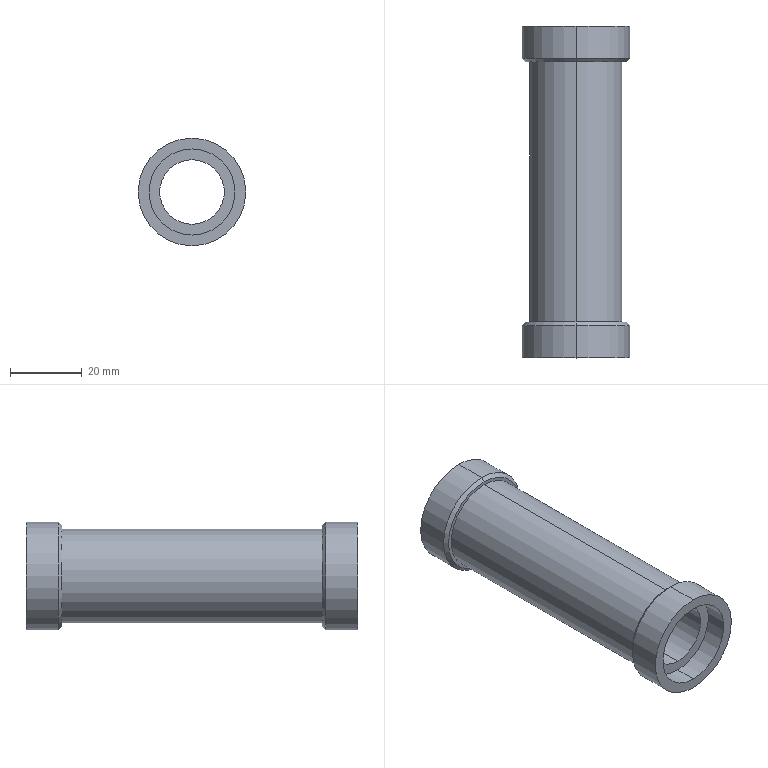Part | STEP file | 2012 Guide shaft | 1 solid | 22 faces | box 30 x 92.5 x 30 mm | volume 26584 mm3 | cylinder 12 | plane 6 | cone 4 | commonest cylinder face diameters 24 x4 30 x4 18 x2 26 x2
STEP:
#1=CARTESIAN_POINT('',(0.,0.,0.));
#2=DIRECTION('',(0.,0.,1.));
#3=DIRECTION('',(1.,0.,0.));
#4=AXIS2_PLACEMENT_3D('',#1,#2,#3);
#5=CARTESIAN_POINT('',(0.,82.5,-14.));
#6=VERTEX_POINT('',#5);
#7=CARTESIAN_POINT('',(0.,82.5,14.));
#8=VERTEX_POINT('',#7);
#9=CARTESIAN_POINT('',(0.,82.5,0.));
#10=DIRECTION('',(0.,-1.,0.));
#11=DIRECTION('',(0.,0.,-1.));
#12=AXIS2_PLACEMENT_3D('',#9,#10,#11);
#13=CIRCLE('',#12,14.);
#14=CARTESIAN_POINT('',(0.,82.5,0.));
#15=DIRECTION('',(0.,1.,0.));
#16=DIRECTION('',(0.,0.,1.));
#17=AXIS2_PLACEMENT_3D('',#14,#15,#16);
#18=CONICAL_SURFACE('',#17,14.,0.7854);
#19=CARTESIAN_POINT('',(3.142,0.));
#20=DIRECTION('',(-1.,0.));
#21=VECTOR('',#20,1.);
#22=LINE('',#19,#21);
#23=(GEOMETRIC_REPRESENTATION_CONTEXT(2)PARAMETRIC_REPRESENTATION_CONTEXT()REPRESENTATION_CONTEXT('',''));
#24=DEFINITIONAL_REPRESENTATION('',(#22),#23);
#25=PCURVE('',#18,#24);
#26=CARTESIAN_POINT('',(15.,82.5,0.));
#27=DIRECTION('',(0.,-1.,0.));
#28=DIRECTION('',(0.,0.,-1.));
#29=AXIS2_PLACEMENT_3D('',#26,#27,#28);
#30=PLANE('',#29);
#31=CARTESIAN_POINT('',(0.,-15.));
#32=DIRECTION('',(1.,0.));
#33=AXIS2_PLACEMENT_2D('',#31,#32);
#34=CIRCLE('',#33,14.);
#35=(GEOMETRIC_REPRESENTATION_CONTEXT(2)PARAMETRIC_REPRESENTATION_CONTEXT()REPRESENTATION_CONTEXT('',''));
#36=DEFINITIONAL_REPRESENTATION('',(#34),#35);
#37=PCURVE('',#30,#36);
#38=SURFACE_CURVE('',#13,(#25,#37),.PCURVE_S1.);
#39=EDGE_CURVE('',#6,#8,#38,.T.);
#40=ORIENTED_EDGE('',*,*,#39,.F.);
#41=CARTESIAN_POINT('',(0.,83.5,-15.));
#42=VERTEX_POINT('',#41);
#43=CARTESIAN_POINT('',(0.,82.5,-14.));
#44=DIRECTION('',(0.,0.7071,-0.7071));
#45=VECTOR('',#44,1.);
#46=LINE('',#43,#45);
#47=CARTESIAN_POINT('',(3.142,0.));
#48=DIRECTION('',(0.,1.));
#49=VECTOR('',#48,1.);
#50=LINE('',#47,#49);
#51=(GEOMETRIC_REPRESENTATION_CONTEXT(2)PARAMETRIC_REPRESENTATION_CONTEXT()REPRESENTATION_CONTEXT('',''));
#52=DEFINITIONAL_REPRESENTATION('',(#50),#51);
#53=PCURVE('',#18,#52);
#54=CARTESIAN_POINT('',(0.,82.5,0.));
#55=DIRECTION('',(0.,1.,0.));
#56=DIRECTION('',(0.,0.,1.));
#57=AXIS2_PLACEMENT_3D('',#54,#55,#56);
#58=CONICAL_SURFACE('',#57,14.,0.7854);
#59=CARTESIAN_POINT('',(3.142,0.));
#60=DIRECTION('',(0.,1.));
#61=VECTOR('',#60,1.);
#62=LINE('',#59,#61);
#63=(GEOMETRIC_REPRESENTATION_CONTEXT(2)PARAMETRIC_REPRESENTATION_CONTEXT()REPRESENTATION_CONTEXT('',''));
#64=DEFINITIONAL_REPRESENTATION('',(#62),#63);
#65=PCURVE('',#58,#64);
#66=SURFACE_CURVE('',#46,(#53,#65),.PCURVE_S1.);
#67=EDGE_CURVE('',#6,#42,#66,.T.);
#68=ORIENTED_EDGE('',*,*,#67,.T.);
#69=CARTESIAN_POINT('',(0.,83.5,15.));
#70=VERTEX_POINT('',#69);
#71=CARTESIAN_POINT('',(0.,83.5,0.));
#72=DIRECTION('',(0.,1.,0.));
#73=DIRECTION('',(0.,0.,-1.));
#74=AXIS2_PLACEMENT_3D('',#71,#72,#73);
#75=CIRCLE('',#74,15.);
#76=CARTESIAN_POINT('',(-3.142,1.));
#77=DIRECTION('',(1.,0.));
#78=VECTOR('',#77,1.);
#79=LINE('',#76,#78);
#80=(GEOMETRIC_REPRESENTATION_CONTEXT(2)PARAMETRIC_REPRESENTATION_CONTEXT()REPRESENTATION_CONTEXT('',''));
#81=DEFINITIONAL_REPRESENTATION('',(#79),#80);
#82=PCURVE('',#18,#81);
#83=CARTESIAN_POINT('',(0.,0.,0.));
#84=DIRECTION('',(0.,-1.,0.));
#85=DIRECTION('',(0.,0.,-1.));
#86=AXIS2_PLACEMENT_3D('',#83,#84,#85);
#87=CYLINDRICAL_SURFACE('',#86,15.);
#88=CARTESIAN_POINT('',(6.283,-83.5));
#89=DIRECTION('',(-1.,0.));
#90=VECTOR('',#89,1.);
#91=LINE('',#88,#90);
#92=(GEOMETRIC_REPRESENTATION_CONTEXT(2)PARAMETRIC_REPRESENTATION_CONTEXT()REPRESENTATION_CONTEXT('',''));
#93=DEFINITIONAL_REPRESENTATION('',(#91),#92);
#94=PCURVE('',#87,#93);
#95=SURFACE_CURVE('',#75,(#82,#94),.PCURVE_S1.);
#96=EDGE_CURVE('',#70,#42,#95,.T.);
#97=ORIENTED_EDGE('',*,*,#96,.F.);
#98=CARTESIAN_POINT('',(0.,82.5,14.));
#99=DIRECTION('',(0.,0.7071,0.7071));
#100=VECTOR('',#99,1.);
#101=LINE('',#98,#100);
#102=CARTESIAN_POINT('',(0.,0.));
#103=DIRECTION('',(0.,1.));
#104=VECTOR('',#103,1.);
#105=LINE('',#102,#104);
#106=(GEOMETRIC_REPRESENTATION_CONTEXT(2)PARAMETRIC_REPRESENTATION_CONTEXT()REPRESENTATION_CONTEXT('',''));
#107=DEFINITIONAL_REPRESENTATION('',(#105),#106);
#108=PCURVE('',#18,#107);
#109=CARTESIAN_POINT('',(6.283,0.));
#110=DIRECTION('',(0.,1.));
#111=VECTOR('',#110,1.);
#112=LINE('',#109,#111);
#113=(GEOMETRIC_REPRESENTATION_CONTEXT(2)PARAMETRIC_REPRESENTATION_CONTEXT()REPRESENTATION_CONTEXT('',''));
#114=DEFINITIONAL_REPRESENTATION('',(#112),#113);
#115=PCURVE('',#58,#114);
#116=SURFACE_CURVE('',#101,(#108,#115),.PCURVE_S1.);
#117=EDGE_CURVE('',#8,#70,#116,.T.);
#118=ORIENTED_EDGE('',*,*,#117,.F.);
#119=EDGE_LOOP('',(#40,#68,#97,#118));
#120=FACE_BOUND('',#119,.T.);
#121=ADVANCED_FACE('',(#120),#18,.T.);
#122=CARTESIAN_POINT('',(0.,10.,14.));
#123=VERTEX_POINT('',#122);
#124=CARTESIAN_POINT('',(0.,10.,-14.));
#125=VERTEX_POINT('',#124);
#126=CARTESIAN_POINT('',(0.,10.,0.));
#127=DIRECTION('',(0.,1.,0.));
#128=DIRECTION('',(0.,0.,1.));
#129=AXIS2_PLACEMENT_3D('',#126,#127,#128);
#130=CIRCLE('',#129,14.);
#131=CARTESIAN_POINT('',(0.,9.,0.));
#132=DIRECTION('',(0.,-1.,0.));
#133=DIRECTION('',(0.,0.,-1.));
#134=AXIS2_PLACEMENT_3D('',#131,#132,#133);
#135=CONICAL_SURFACE('',#134,15.,0.7854);
#136=CARTESIAN_POINT('',(3.142,-1.));
#137=DIRECTION('',(-1.,0.));
#138=VECTOR('',#137,1.);
#139=LINE('',#136,#138);
#140=(GEOMETRIC_REPRESENTATION_CONTEXT(2)PARAMETRIC_REPRESENTATION_CONTEXT()REPRESENTATION_CONTEXT('',''));
#141=DEFINITIONAL_REPRESENTATION('',(#139),#140);
#142=PCURVE('',#135,#141);
#143=CARTESIAN_POINT('',(13.,10.,0.));
#144=DIRECTION('',(0.,1.,0.));
#145=DIRECTION('',(0.,0.,1.));
#146=AXIS2_PLACEMENT_3D('',#143,#144,#145);
#147=PLANE('',#146);
#148=CARTESIAN_POINT('',(0.,-13.));
#149=DIRECTION('',(1.,0.));
#150=AXIS2_PLACEMENT_2D('',#148,#149);
#151=CIRCLE('',#150,14.);
#152=(GEOMETRIC_REPRESENTATION_CONTEXT(2)PARAMETRIC_REPRESENTATION_CONTEXT()REPRESENTATION_CONTEXT('',''));
#153=DEFINITIONAL_REPRESENTATION('',(#151),#152);
#154=PCURVE('',#147,#153);
#155=SURFACE_CURVE('',#130,(#142,#154),.PCURVE_S1.);
#156=EDGE_CURVE('',#123,#125,#155,.T.);
#157=ORIENTED_EDGE('',*,*,#156,.F.);
#158=CARTESIAN_POINT('',(0.,9.,15.));
#159=VERTEX_POINT('',#158);
#160=CARTESIAN_POINT('',(0.,9.,15.));
#161=DIRECTION('',(0.,-0.7071,0.7071));
#162=VECTOR('',#161,1.);
#163=LINE('',#160,#162);
#164=CARTESIAN_POINT('',(3.142,0.));
#165=DIRECTION('',(0.,1.));
#166=VECTOR('',#165,1.);
#167=LINE('',#164,#166);
#168=(GEOMETRIC_REPRESENTATION_CONTEXT(2)PARAMETRIC_REPRESENTATION_CONTEXT()REPRESENTATION_CONTEXT('',''));
#169=DEFINITIONAL_REPRESENTATION('',(#167),#168);
#170=PCURVE('',#135,#169);
#171=CARTESIAN_POINT('',(0.,9.,0.));
#172=DIRECTION('',(0.,-1.,0.));
#173=DIRECTION('',(0.,0.,-1.));
#174=AXIS2_PLACEMENT_3D('',#171,#172,#173);
#175=CONICAL_SURFACE('',#174,15.,0.7854);
#176=CARTESIAN_POINT('',(3.142,0.));
#177=DIRECTION('',(0.,1.));
#178=VECTOR('',#177,1.);
#179=LINE('',#176,#178);
#180=(GEOMETRIC_REPRESENTATION_CONTEXT(2)PARAMETRIC_REPRESENTATION_CONTEXT()REPRESENTATION_CONTEXT('',''));
#181=DEFINITIONAL_REPRESENTATION('',(#179),#180);
#182=PCURVE('',#175,#181);
#183=SURFACE_CURVE('',#163,(#170,#182),.PCURVE_S1.);
#184=EDGE_CURVE('',#123,#159,#183,.T.);
#185=ORIENTED_EDGE('',*,*,#184,.T.);
#186=CARTESIAN_POINT('',(0.,9.,-15.));
#187=VERTEX_POINT('',#186);
#188=CARTESIAN_POINT('',(0.,9.,0.));
#189=DIRECTION('',(0.,-1.,0.));
#190=DIRECTION('',(0.,0.,1.));
#191=AXIS2_PLACEMENT_3D('',#188,#189,#190);
#192=CIRCLE('',#191,15.);
#193=CARTESIAN_POINT('',(-3.142,0.));
#194=DIRECTION('',(1.,0.));
#195=VECTOR('',#194,1.);
#196=LINE('',#193,#195);
#197=(GEOMETRIC_REPRESENTATION_CONTEXT(2)PARAMETRIC_REPRESENTATION_CONTEXT()REPRESENTATION_CONTEXT('',''));
#198=DEFINITIONAL_REPRESENTATION('',(#196),#197);
#199=PCURVE('',#135,#198);
#200=CARTESIAN_POINT('',(0.,0.,0.));
#201=DIRECTION('',(0.,-1.,0.));
#202=DIRECTION('',(0.,0.,-1.));
#203=AXIS2_PLACEMENT_3D('',#200,#201,#202);
#204=CYLINDRICAL_SURFACE('',#203,15.);
#205=CARTESIAN_POINT('',(-3.142,-9.));
#206=DIRECTION('',(1.,0.));
#207=VECTOR('',#206,1.);
#208=LINE('',#205,#207);
#209=(GEOMETRIC_REPRESENTATION_CONTEXT(2)PARAMETRIC_REPRESENTATION_CONTEXT()REPRESENTATION_CONTEXT('',''));
#210=DEFINITIONAL_REPRESENTATION('',(#208),#209);
#211=PCURVE('',#204,#210);
#212=SURFACE_CURVE('',#192,(#199,#211),.PCURVE_S1.);
#213=EDGE_CURVE('',#187,#159,#212,.T.);
#214=ORIENTED_EDGE('',*,*,#213,.F.);
#215=CARTESIAN_POINT('',(0.,9.,-15.));
#216=DIRECTION('',(0.,-0.7071,-0.7071));
#217=VECTOR('',#216,1.);
#218=LINE('',#215,#217);
#219=CARTESIAN_POINT('',(0.,0.));
#220=DIRECTION('',(0.,1.));
#221=VECTOR('',#220,1.);
#222=LINE('',#219,#221);
#223=(GEOMETRIC_REPRESENTATION_CONTEXT(2)PARAMETRIC_REPRESENTATION_CONTEXT()REPRESENTATION_CONTEXT('',''));
#224=DEFINITIONAL_REPRESENTATION('',(#222),#223);
#225=PCURVE('',#135,#224);
#226=CARTESIAN_POINT('',(6.283,0.));
#227=DIRECTION('',(0.,1.));
#228=VECTOR('',#227,1.);
#229=LINE('',#226,#228);
#230=(GEOMETRIC_REPRESENTATION_CONTEXT(2)PARAMETRIC_REPRESENTATION_CONTEXT()REPRESENTATION_CONTEXT('',''));
#231=DEFINITIONAL_REPRESENTATION('',(#229),#230);
#232=PCURVE('',#175,#231);
#233=SURFACE_CURVE('',#218,(#225,#232),.PCURVE_S1.);
#234=EDGE_CURVE('',#125,#187,#233,.T.);
#235=ORIENTED_EDGE('',*,*,#234,.F.);
#236=EDGE_LOOP('',(#157,#185,#214,#235));
#237=FACE_BOUND('',#236,.T.);
#238=ADVANCED_FACE('',(#237),#135,.T.);
#239=CARTESIAN_POINT('',(0.,86.4,-9.));
#240=VERTEX_POINT('',#239);
#241=CARTESIAN_POINT('',(0.,6.1,-9.));
#242=VERTEX_POINT('',#241);
#243=CARTESIAN_POINT('',(0.,92.5,-9.));
#244=DIRECTION('',(0.,-1.,0.));
#245=VECTOR('',#244,1.);
#246=LINE('',#243,#245);
#247=CARTESIAN_POINT('',(0.,92.5,0.));
#248=DIRECTION('',(0.,-1.,0.));
#249=DIRECTION('',(0.,0.,-1.));
#250=AXIS2_PLACEMENT_3D('',#247,#248,#249);
#251=CYLINDRICAL_SURFACE('',#250,9.);
#252=CARTESIAN_POINT('',(6.283,0.));
#253=DIRECTION('',(0.,1.));
#254=VECTOR('',#253,1.);
#255=LINE('',#252,#254);
#256=(GEOMETRIC_REPRESENTATION_CONTEXT(2)PARAMETRIC_REPRESENTATION_CONTEXT()REPRESENTATION_CONTEXT('',''));
#257=DEFINITIONAL_REPRESENTATION('',(#255),#256);
#258=PCURVE('',#251,#257);
#259=CARTESIAN_POINT('',(0.,92.5,0.));
#260=DIRECTION('',(0.,-1.,0.));
#261=DIRECTION('',(0.,0.,-1.));
#262=AXIS2_PLACEMENT_3D('',#259,#260,#261);
#263=CYLINDRICAL_SURFACE('',#262,9.);
#264=CARTESIAN_POINT('',(0.,0.));
#265=DIRECTION('',(0.,1.));
#266=VECTOR('',#265,1.);
#267=LINE('',#264,#266);
#268=(GEOMETRIC_REPRESENTATION_CONTEXT(2)PARAMETRIC_REPRESENTATION_CONTEXT()REPRESENTATION_CONTEXT('',''));
#269=DEFINITIONAL_REPRESENTATION('',(#267),#268);
#270=PCURVE('',#263,#269);
#271=SURFACE_CURVE('',#246,(#258,#270),.PCURVE_S1.);
#272=EDGE_CURVE('',#240,#242,#271,.T.);
#273=ORIENTED_EDGE('',*,*,#272,.T.);
#274=CARTESIAN_POINT('',(0.,6.1,9.));
#275=VERTEX_POINT('',#274);
#276=CARTESIAN_POINT('',(0.,6.1,0.));
#277=DIRECTION('',(0.,-1.,0.));
#278=DIRECTION('',(0.,0.,-1.));
#279=AXIS2_PLACEMENT_3D('',#276,#277,#278);
#280=CIRCLE('',#279,9.);
#281=CARTESIAN_POINT('',(0.,86.4));
#282=DIRECTION('',(1.,0.));
#283=VECTOR('',#282,1.);
#284=LINE('',#281,#283);
#285=(GEOMETRIC_REPRESENTATION_CONTEXT(2)PARAMETRIC_REPRESENTATION_CONTEXT()REPRESENTATION_CONTEXT('',''));
#286=DEFINITIONAL_REPRESENTATION('',(#284),#285);
#287=PCURVE('',#251,#286);
#288=CARTESIAN_POINT('',(0.,6.1,0.));
#289=DIRECTION('',(0.,-1.,0.));
#290=DIRECTION('',(0.,0.,-1.));
#291=AXIS2_PLACEMENT_3D('',#288,#289,#290);
#292=PLANE('',#291);
#293=CARTESIAN_POINT('',(0.,0.));
#294=DIRECTION('',(1.,0.));
#295=AXIS2_PLACEMENT_2D('',#293,#294);
#296=CIRCLE('',#295,9.);
#297=(GEOMETRIC_REPRESENTATION_CONTEXT(2)PARAMETRIC_REPRESENTATION_CONTEXT()REPRESENTATION_CONTEXT('',''));
#298=DEFINITIONAL_REPRESENTATION('',(#296),#297);
#299=PCURVE('',#292,#298);
#300=SURFACE_CURVE('',#280,(#287,#299),.PCURVE_S1.);
#301=EDGE_CURVE('',#275,#242,#300,.T.);
#302=ORIENTED_EDGE('',*,*,#301,.F.);
#303=CARTESIAN_POINT('',(0.,86.4,9.));
#304=VERTEX_POINT('',#303);
#305=CARTESIAN_POINT('',(0.,92.5,9.));
#306=DIRECTION('',(0.,-1.,0.));
#307=VECTOR('',#306,1.);
#308=LINE('',#305,#307);
#309=CARTESIAN_POINT('',(3.142,0.));
#310=DIRECTION('',(0.,1.));
#311=VECTOR('',#310,1.);
#312=LINE('',#309,#311);
#313=(GEOMETRIC_REPRESENTATION_CONTEXT(2)PARAMETRIC_REPRESENTATION_CONTEXT()REPRESENTATION_CONTEXT('',''));
#314=DEFINITIONAL_REPRESENTATION('',(#312),#313);
#315=PCURVE('',#251,#314);
#316=CARTESIAN_POINT('',(3.142,0.));
#317=DIRECTION('',(0.,1.));
#318=VECTOR('',#317,1.);
#319=LINE('',#316,#318);
#320=(GEOMETRIC_REPRESENTATION_CONTEXT(2)PARAMETRIC_REPRESENTATION_CONTEXT()REPRESENTATION_CONTEXT('',''));
#321=DEFINITIONAL_REPRESENTATION('',(#319),#320);
#322=PCURVE('',#263,#321);
#323=SURFACE_CURVE('',#308,(#315,#322),.PCURVE_S1.);
#324=EDGE_CURVE('',#304,#275,#323,.T.);
#325=ORIENTED_EDGE('',*,*,#324,.F.);
#326=CARTESIAN_POINT('',(0.,86.4,0.));
#327=DIRECTION('',(0.,1.,0.));
#328=DIRECTION('',(0.,0.,1.));
#329=AXIS2_PLACEMENT_3D('',#326,#327,#328);
#330=CIRCLE('',#329,9.);
#331=CARTESIAN_POINT('',(9.425,6.1));
#332=DIRECTION('',(-1.,0.));
#333=VECTOR('',#332,1.);
#334=LINE('',#331,#333);
#335=(GEOMETRIC_REPRESENTATION_CONTEXT(2)PARAMETRIC_REPRESENTATION_CONTEXT()REPRESENTATION_CONTEXT('',''));
#336=DEFINITIONAL_REPRESENTATION('',(#334),#335);
#337=PCURVE('',#251,#336);
#338=CARTESIAN_POINT('',(0.,86.4,0.));
#339=DIRECTION('',(0.,1.,0.));
#340=DIRECTION('',(0.,0.,1.));
#341=AXIS2_PLACEMENT_3D('',#338,#339,#340);
#342=PLANE('',#341);
#343=CARTESIAN_POINT('',(0.,0.));
#344=DIRECTION('',(1.,0.));
#345=AXIS2_PLACEMENT_2D('',#343,#344);
#346=CIRCLE('',#345,9.);
#347=(GEOMETRIC_REPRESENTATION_CONTEXT(2)PARAMETRIC_REPRESENTATION_CONTEXT()REPRESENTATION_CONTEXT('',''));
#348=DEFINITIONAL_REPRESENTATION('',(#346),#347);
#349=PCURVE('',#342,#348);
#350=SURFACE_CURVE('',#330,(#337,#349),.PCURVE_S1.);
#351=EDGE_CURVE('',#240,#304,#350,.T.);
#352=ORIENTED_EDGE('',*,*,#351,.F.);
#353=EDGE_LOOP('',(#273,#302,#325,#352));
#354=FACE_BOUND('',#353,.F.);
#355=ADVANCED_FACE('',(#354),#251,.F.);
#356=CARTESIAN_POINT('',(0.,86.4,12.));
#357=VERTEX_POINT('',#356);
#358=CARTESIAN_POINT('',(0.,92.5,12.));
#359=VERTEX_POINT('',#358);
#360=CARTESIAN_POINT('',(0.,86.4,12.));
#361=DIRECTION('',(0.,1.,0.));
#362=VECTOR('',#361,1.);
#363=LINE('',#360,#362);
#364=CARTESIAN_POINT('',(0.,86.4,0.));
#365=DIRECTION('',(0.,1.,0.));
#366=DIRECTION('',(0.,0.,1.));
#367=AXIS2_PLACEMENT_3D('',#364,#365,#366);
#368=CYLINDRICAL_SURFACE('',#367,12.);
#369=CARTESIAN_POINT('',(6.283,0.));
#370=DIRECTION('',(0.,1.));
#371=VECTOR('',#370,1.);
#372=LINE('',#369,#371);
#373=(GEOMETRIC_REPRESENTATION_CONTEXT(2)PARAMETRIC_REPRESENTATION_CONTEXT()REPRESENTATION_CONTEXT('',''));
#374=DEFINITIONAL_REPRESENTATION('',(#372),#373);
#375=PCURVE('',#368,#374);
#376=CARTESIAN_POINT('',(0.,86.4,0.));
#377=DIRECTION('',(0.,1.,0.));
#378=DIRECTION('',(0.,0.,1.));
#379=AXIS2_PLACEMENT_3D('',#376,#377,#378);
#380=CYLINDRICAL_SURFACE('',#379,12.);
#381=CARTESIAN_POINT('',(0.,0.));
#382=DIRECTION('',(0.,1.));
#383=VECTOR('',#382,1.);
#384=LINE('',#381,#383);
#385=(GEOMETRIC_REPRESENTATION_CONTEXT(2)PARAMETRIC_REPRESENTATION_CONTEXT()REPRESENTATION_CONTEXT('',''));
#386=DEFINITIONAL_REPRESENTATION('',(#384),#385);
#387=PCURVE('',#380,#386);
#388=SURFACE_CURVE('',#363,(#375,#387),.PCURVE_S1.);
#389=EDGE_CURVE('',#357,#359,#388,.T.);
#390=ORIENTED_EDGE('',*,*,#389,.T.);
#391=CARTESIAN_POINT('',(0.,92.5,-12.));
#392=VERTEX_POINT('',#391);
#393=CARTESIAN_POINT('',(0.,92.5,0.));
#394=DIRECTION('',(0.,1.,0.));
#395=DIRECTION('',(0.,0.,1.));
#396=AXIS2_PLACEMENT_3D('',#393,#394,#395);
#397=CIRCLE('',#396,12.);
#398=CARTESIAN_POINT('',(0.,6.1));
#399=DIRECTION('',(1.,0.));
#400=VECTOR('',#399,1.);
#401=LINE('',#398,#400);
#402=(GEOMETRIC_REPRESENTATION_CONTEXT(2)PARAMETRIC_REPRESENTATION_CONTEXT()REPRESENTATION_CONTEXT('',''));
#403=DEFINITIONAL_REPRESENTATION('',(#401),#402);
#404=PCURVE('',#368,#403);
#405=CARTESIAN_POINT('',(0.,92.5,0.));
#406=DIRECTION('',(0.,1.,0.));
#407=DIRECTION('',(0.,0.,1.));
#408=AXIS2_PLACEMENT_3D('',#405,#406,#407);
#409=PLANE('',#408);
#410=CARTESIAN_POINT('',(0.,0.));
#411=DIRECTION('',(1.,0.));
#412=AXIS2_PLACEMENT_2D('',#410,#411);
#413=CIRCLE('',#412,12.);
#414=(GEOMETRIC_REPRESENTATION_CONTEXT(2)PARAMETRIC_REPRESENTATION_CONTEXT()REPRESENTATION_CONTEXT('',''));
#415=DEFINITIONAL_REPRESENTATION('',(#413),#414);
#416=PCURVE('',#409,#415);
#417=SURFACE_CURVE('',#397,(#404,#416),.PCURVE_S1.);
#418=EDGE_CURVE('',#392,#359,#417,.T.);
#419=ORIENTED_EDGE('',*,*,#418,.F.);
#420=CARTESIAN_POINT('',(0.,86.4,-12.));
#421=VERTEX_POINT('',#420);
#422=CARTESIAN_POINT('',(0.,86.4,-12.));
#423=DIRECTION('',(0.,1.,0.));
#424=VECTOR('',#423,1.);
#425=LINE('',#422,#424);
#426=CARTESIAN_POINT('',(3.142,0.));
#427=DIRECTION('',(0.,1.));
#428=VECTOR('',#427,1.);
#429=LINE('',#426,#428);
#430=(GEOMETRIC_REPRESENTATION_CONTEXT(2)PARAMETRIC_REPRESENTATION_CONTEXT()REPRESENTATION_CONTEXT('',''));
#431=DEFINITIONAL_REPRESENTATION('',(#429),#430);
#432=PCURVE('',#368,#431);
#433=CARTESIAN_POINT('',(3.142,0.));
#434=DIRECTION('',(0.,1.));
#435=VECTOR('',#434,1.);
#436=LINE('',#433,#435);
#437=(GEOMETRIC_REPRESENTATION_CONTEXT(2)PARAMETRIC_REPRESENTATION_CONTEXT()REPRESENTATION_CONTEXT('',''));
#438=DEFINITIONAL_REPRESENTATION('',(#436),#437);
#439=PCURVE('',#380,#438);
#440=SURFACE_CURVE('',#425,(#432,#439),.PCURVE_S1.);
#441=EDGE_CURVE('',#421,#392,#440,.T.);
#442=ORIENTED_EDGE('',*,*,#441,.F.);
#443=CARTESIAN_POINT('',(0.,86.4,0.));
#444=DIRECTION('',(0.,1.,0.));
#445=DIRECTION('',(0.,0.,1.));
#446=AXIS2_PLACEMENT_3D('',#443,#444,#445);
#447=CIRCLE('',#446,12.);
#448=CARTESIAN_POINT('',(0.,0.));
#449=DIRECTION('',(1.,0.));
#450=VECTOR('',#449,1.);
#451=LINE('',#448,#450);
#452=(GEOMETRIC_REPRESENTATION_CONTEXT(2)PARAMETRIC_REPRESENTATION_CONTEXT()REPRESENTATION_CONTEXT('',''));
#453=DEFINITIONAL_REPRESENTATION('',(#451),#452);
#454=PCURVE('',#368,#453);
#455=CARTESIAN_POINT('',(0.,0.));
#456=DIRECTION('',(1.,0.));
#457=AXIS2_PLACEMENT_2D('',#455,#456);
#458=CIRCLE('',#457,12.);
#459=(GEOMETRIC_REPRESENTATION_CONTEXT(2)PARAMETRIC_REPRESENTATION_CONTEXT()REPRESENTATION_CONTEXT('',''));
#460=DEFINITIONAL_REPRESENTATION('',(#458),#459);
#461=PCURVE('',#342,#460);
#462=SURFACE_CURVE('',#447,(#454,#461),.PCURVE_S1.);
#463=EDGE_CURVE('',#421,#357,#462,.T.);
#464=ORIENTED_EDGE('',*,*,#463,.T.);
#465=EDGE_LOOP('',(#390,#419,#442,#464));
#466=FACE_BOUND('',#465,.F.);
#467=ADVANCED_FACE('',(#466),#368,.F.);
#468=CARTESIAN_POINT('',(0.,6.1,-12.));
#469=VERTEX_POINT('',#468);
#470=CARTESIAN_POINT('',(0.,0.,-12.));
#471=VERTEX_POINT('',#470);
#472=CARTESIAN_POINT('',(0.,6.1,-12.));
#473=DIRECTION('',(0.,-1.,0.));
#474=VECTOR('',#473,1.);
#475=LINE('',#472,#474);
#476=CARTESIAN_POINT('',(0.,6.1,0.));
#477=DIRECTION('',(0.,-1.,0.));
#478=DIRECTION('',(0.,0.,-1.));
#479=AXIS2_PLACEMENT_3D('',#476,#477,#478);
#480=CYLINDRICAL_SURFACE('',#479,12.);
#481=CARTESIAN_POINT('',(6.283,0.));
#482=DIRECTION('',(0.,1.));
#483=VECTOR('',#482,1.);
#484=LINE('',#481,#483);
#485=(GEOMETRIC_REPRESENTATION_CONTEXT(2)PARAMETRIC_REPRESENTATION_CONTEXT()REPRESENTATION_CONTEXT('',''));
#486=DEFINITIONAL_REPRESENTATION('',(#484),#485);
#487=PCURVE('',#480,#486);
#488=CARTESIAN_POINT('',(0.,6.1,0.));
#489=DIRECTION('',(0.,-1.,0.));
#490=DIRECTION('',(0.,0.,-1.));
#491=AXIS2_PLACEMENT_3D('',#488,#489,#490);
#492=CYLINDRICAL_SURFACE('',#491,12.);
#493=CARTESIAN_POINT('',(0.,0.));
#494=DIRECTION('',(0.,1.));
#495=VECTOR('',#494,1.);
#496=LINE('',#493,#495);
#497=(GEOMETRIC_REPRESENTATION_CONTEXT(2)PARAMETRIC_REPRESENTATION_CONTEXT()REPRESENTATION_CONTEXT('',''));
#498=DEFINITIONAL_REPRESENTATION('',(#496),#497);
#499=PCURVE('',#492,#498);
#500=SURFACE_CURVE('',#475,(#487,#499),.PCURVE_S1.);
#501=EDGE_CURVE('',#469,#471,#500,.T.);
#502=ORIENTED_EDGE('',*,*,#501,.T.);
#503=CARTESIAN_POINT('',(0.,0.,12.));
#504=VERTEX_POINT('',#503);
#505=CARTESIAN_POINT('',(0.,0.,0.));
#506=DIRECTION('',(0.,-1.,0.));
#507=DIRECTION('',(0.,0.,-1.));
#508=AXIS2_PLACEMENT_3D('',#505,#506,#507);
#509=CIRCLE('',#508,12.);
#510=CARTESIAN_POINT('',(0.,6.1));
#511=DIRECTION('',(1.,0.));
#512=VECTOR('',#511,1.);
#513=LINE('',#510,#512);
#514=(GEOMETRIC_REPRESENTATION_CONTEXT(2)PARAMETRIC_REPRESENTATION_CONTEXT()REPRESENTATION_CONTEXT('',''));
#515=DEFINITIONAL_REPRESENTATION('',(#513),#514);
#516=PCURVE('',#480,#515);
#517=CARTESIAN_POINT('',(15.,0.,0.));
#518=DIRECTION('',(0.,-1.,0.));
#519=DIRECTION('',(0.,0.,-1.));
#520=AXIS2_PLACEMENT_3D('',#517,#518,#519);
#521=PLANE('',#520);
#522=CARTESIAN_POINT('',(0.,-15.));
#523=DIRECTION('',(1.,0.));
#524=AXIS2_PLACEMENT_2D('',#522,#523);
#525=CIRCLE('',#524,12.);
#526=(GEOMETRIC_REPRESENTATION_CONTEXT(2)PARAMETRIC_REPRESENTATION_CONTEXT()REPRESENTATION_CONTEXT('',''));
#527=DEFINITIONAL_REPRESENTATION('',(#525),#526);
#528=PCURVE('',#521,#527);
#529=SURFACE_CURVE('',#509,(#516,#528),.PCURVE_S1.);
#530=EDGE_CURVE('',#504,#471,#529,.T.);
#531=ORIENTED_EDGE('',*,*,#530,.F.);
#532=CARTESIAN_POINT('',(0.,6.1,12.));
#533=VERTEX_POINT('',#532);
#534=CARTESIAN_POINT('',(0.,6.1,12.));
#535=DIRECTION('',(0.,-1.,0.));
#536=VECTOR('',#535,1.);
#537=LINE('',#534,#536);
#538=CARTESIAN_POINT('',(3.142,0.));
#539=DIRECTION('',(0.,1.));
#540=VECTOR('',#539,1.);
#541=LINE('',#538,#540);
#542=(GEOMETRIC_REPRESENTATION_CONTEXT(2)PARAMETRIC_REPRESENTATION_CONTEXT()REPRESENTATION_CONTEXT('',''));
#543=DEFINITIONAL_REPRESENTATION('',(#541),#542);
#544=PCURVE('',#480,#543);
#545=CARTESIAN_POINT('',(3.142,0.));
#546=DIRECTION('',(0.,1.));
#547=VECTOR('',#546,1.);
#548=LINE('',#545,#547);
#549=(GEOMETRIC_REPRESENTATION_CONTEXT(2)PARAMETRIC_REPRESENTATION_CONTEXT()REPRESENTATION_CONTEXT('',''));
#550=DEFINITIONAL_REPRESENTATION('',(#548),#549);
#551=PCURVE('',#492,#550);
#552=SURFACE_CURVE('',#537,(#544,#551),.PCURVE_S1.);
#553=EDGE_CURVE('',#533,#504,#552,.T.);
#554=ORIENTED_EDGE('',*,*,#553,.F.);
#555=CARTESIAN_POINT('',(0.,6.1,0.));
#556=DIRECTION('',(0.,-1.,0.));
#557=DIRECTION('',(0.,0.,-1.));
#558=AXIS2_PLACEMENT_3D('',#555,#556,#557);
#559=CIRCLE('',#558,12.);
#560=CARTESIAN_POINT('',(0.,0.));
#561=DIRECTION('',(1.,0.));
#562=VECTOR('',#561,1.);
#563=LINE('',#560,#562);
#564=(GEOMETRIC_REPRESENTATION_CONTEXT(2)PARAMETRIC_REPRESENTATION_CONTEXT()REPRESENTATION_CONTEXT('',''));
#565=DEFINITIONAL_REPRESENTATION('',(#563),#564);
#566=PCURVE('',#480,#565);
#567=CARTESIAN_POINT('',(0.,0.));
#568=DIRECTION('',(1.,0.));
#569=AXIS2_PLACEMENT_2D('',#567,#568);
#570=CIRCLE('',#569,12.);
#571=(GEOMETRIC_REPRESENTATION_CONTEXT(2)PARAMETRIC_REPRESENTATION_CONTEXT()REPRESENTATION_CONTEXT('',''));
#572=DEFINITIONAL_REPRESENTATION('',(#570),#571);
#573=PCURVE('',#292,#572);
#574=SURFACE_CURVE('',#559,(#566,#573),.PCURVE_S1.);
#575=EDGE_CURVE('',#533,#469,#574,.T.);
#576=ORIENTED_EDGE('',*,*,#575,.T.);
#577=EDGE_LOOP('',(#502,#531,#554,#576));
#578=FACE_BOUND('',#577,.F.);
#579=ADVANCED_FACE('',(#578),#480,.F.);
#580=ORIENTED_EDGE('',*,*,#213,.T.);
#581=CARTESIAN_POINT('',(0.,0.,15.));
#582=VERTEX_POINT('',#581);
#583=CARTESIAN_POINT('',(0.,0.,15.));
#584=DIRECTION('',(0.,-1.,0.));
#585=VECTOR('',#584,1.);
#586=LINE('',#583,#585);
#587=CARTESIAN_POINT('',(3.142,0.));
#588=DIRECTION('',(0.,1.));
#589=VECTOR('',#588,1.);
#590=LINE('',#587,#589);
#591=(GEOMETRIC_REPRESENTATION_CONTEXT(2)PARAMETRIC_REPRESENTATION_CONTEXT()REPRESENTATION_CONTEXT('',''));
#592=DEFINITIONAL_REPRESENTATION('',(#590),#591);
#593=PCURVE('',#204,#592);
#594=CARTESIAN_POINT('',(0.,0.,0.));
#595=DIRECTION('',(0.,-1.,0.));
#596=DIRECTION('',(0.,0.,-1.));
#597=AXIS2_PLACEMENT_3D('',#594,#595,#596);
#598=CYLINDRICAL_SURFACE('',#597,15.);
#599=CARTESIAN_POINT('',(3.142,0.));
#600=DIRECTION('',(0.,1.));
#601=VECTOR('',#600,1.);
#602=LINE('',#599,#601);
#603=(GEOMETRIC_REPRESENTATION_CONTEXT(2)PARAMETRIC_REPRESENTATION_CONTEXT()REPRESENTATION_CONTEXT('',''));
#604=DEFINITIONAL_REPRESENTATION('',(#602),#603);
#605=PCURVE('',#598,#604);
#606=SURFACE_CURVE('',#586,(#593,#605),.PCURVE_S1.);
#607=EDGE_CURVE('',#159,#582,#606,.T.);
#608=ORIENTED_EDGE('',*,*,#607,.T.);
#609=CARTESIAN_POINT('',(0.,0.,-15.));
#610=VERTEX_POINT('',#609);
#611=CARTESIAN_POINT('',(0.,0.,0.));
#612=DIRECTION('',(0.,-1.,0.));
#613=DIRECTION('',(0.,0.,-1.));
#614=AXIS2_PLACEMENT_3D('',#611,#612,#613);
#615=CIRCLE('',#614,15.);
#616=CARTESIAN_POINT('',(0.,0.));
#617=DIRECTION('',(1.,0.));
#618=VECTOR('',#617,1.);
#619=LINE('',#616,#618);
#620=(GEOMETRIC_REPRESENTATION_CONTEXT(2)PARAMETRIC_REPRESENTATION_CONTEXT()REPRESENTATION_CONTEXT('',''));
#621=DEFINITIONAL_REPRESENTATION('',(#619),#620);
#622=PCURVE('',#204,#621);
#623=CARTESIAN_POINT('',(0.,-15.));
#624=DIRECTION('',(1.,0.));
#625=AXIS2_PLACEMENT_2D('',#623,#624);
#626=CIRCLE('',#625,15.);
#627=(GEOMETRIC_REPRESENTATION_CONTEXT(2)PARAMETRIC_REPRESENTATION_CONTEXT()REPRESENTATION_CONTEXT('',''));
#628=DEFINITIONAL_REPRESENTATION('',(#626),#627);
#629=PCURVE('',#521,#628);
#630=SURFACE_CURVE('',#615,(#622,#629),.PCURVE_S1.);
#631=EDGE_CURVE('',#610,#582,#630,.T.);
#632=ORIENTED_EDGE('',*,*,#631,.F.);
#633=CARTESIAN_POINT('',(0.,0.,-15.));
#634=DIRECTION('',(0.,-1.,0.));
#635=VECTOR('',#634,1.);
#636=LINE('',#633,#635);
#637=CARTESIAN_POINT('',(0.,0.));
#638=DIRECTION('',(0.,1.));
#639=VECTOR('',#638,1.);
#640=LINE('',#637,#639);
#641=(GEOMETRIC_REPRESENTATION_CONTEXT(2)PARAMETRIC_REPRESENTATION_CONTEXT()REPRESENTATION_CONTEXT('',''));
#642=DEFINITIONAL_REPRESENTATION('',(#640),#641);
#643=PCURVE('',#204,#642);
#644=CARTESIAN_POINT('',(6.283,0.));
#645=DIRECTION('',(0.,1.));
#646=VECTOR('',#645,1.);
#647=LINE('',#644,#646);
#648=(GEOMETRIC_REPRESENTATION_CONTEXT(2)PARAMETRIC_REPRESENTATION_CONTEXT()REPRESENTATION_CONTEXT('',''));
#649=DEFINITIONAL_REPRESENTATION('',(#647),#648);
#650=PCURVE('',#598,#649);
#651=SURFACE_CURVE('',#636,(#643,#650),.PCURVE_S1.);
#652=EDGE_CURVE('',#187,#610,#651,.T.);
#653=ORIENTED_EDGE('',*,*,#652,.F.);
#654=EDGE_LOOP('',(#580,#608,#632,#653));
#655=FACE_BOUND('',#654,.T.);
#656=ADVANCED_FACE('',(#655),#204,.T.);
#657=CARTESIAN_POINT('',(0.,82.5,-13.));
#658=VERTEX_POINT('',#657);
#659=CARTESIAN_POINT('',(0.,82.5,13.));
#660=VERTEX_POINT('',#659);
#661=CARTESIAN_POINT('',(0.,82.5,0.));
#662=DIRECTION('',(0.,-1.,0.));
#663=DIRECTION('',(0.,0.,-1.));
#664=AXIS2_PLACEMENT_3D('',#661,#662,#663);
#665=CIRCLE('',#664,13.);
#666=CARTESIAN_POINT('',(0.,0.,0.));
#667=DIRECTION('',(0.,-1.,0.));
#668=DIRECTION('',(0.,0.,-1.));
#669=AXIS2_PLACEMENT_3D('',#666,#667,#668);
#670=CYLINDRICAL_SURFACE('',#669,13.);
#671=CARTESIAN_POINT('',(0.,-82.5));
#672=DIRECTION('',(1.,0.));
#673=VECTOR('',#672,1.);
#674=LINE('',#671,#673);
#675=(GEOMETRIC_REPRESENTATION_CONTEXT(2)PARAMETRIC_REPRESENTATION_CONTEXT()REPRESENTATION_CONTEXT('',''));
#676=DEFINITIONAL_REPRESENTATION('',(#674),#675);
#677=PCURVE('',#670,#676);
#678=CARTESIAN_POINT('',(0.,-15.));
#679=DIRECTION('',(1.,0.));
#680=AXIS2_PLACEMENT_2D('',#678,#679);
#681=CIRCLE('',#680,13.);
#682=(GEOMETRIC_REPRESENTATION_CONTEXT(2)PARAMETRIC_REPRESENTATION_CONTEXT()REPRESENTATION_CONTEXT('',''));
#683=DEFINITIONAL_REPRESENTATION('',(#681),#682);
#684=PCURVE('',#30,#683);
#685=SURFACE_CURVE('',#665,(#677,#684),.PCURVE_S1.);
#686=EDGE_CURVE('',#658,#660,#685,.T.);
#687=ORIENTED_EDGE('',*,*,#686,.T.);
#688=CARTESIAN_POINT('',(0.,10.,13.));
#689=VERTEX_POINT('',#688);
#690=CARTESIAN_POINT('',(0.,0.,13.));
#691=DIRECTION('',(0.,-1.,0.));
#692=VECTOR('',#691,1.);
#693=LINE('',#690,#692);
#694=CARTESIAN_POINT('',(3.142,0.));
#695=DIRECTION('',(0.,1.));
#696=VECTOR('',#695,1.);
#697=LINE('',#694,#696);
#698=(GEOMETRIC_REPRESENTATION_CONTEXT(2)PARAMETRIC_REPRESENTATION_CONTEXT()REPRESENTATION_CONTEXT('',''));
#699=DEFINITIONAL_REPRESENTATION('',(#697),#698);
#700=PCURVE('',#670,#699);
#701=CARTESIAN_POINT('',(0.,0.,0.));
#702=DIRECTION('',(0.,-1.,0.));
#703=DIRECTION('',(0.,0.,-1.));
#704=AXIS2_PLACEMENT_3D('',#701,#702,#703);
#705=CYLINDRICAL_SURFACE('',#704,13.);
#706=CARTESIAN_POINT('',(3.142,0.));
#707=DIRECTION('',(0.,1.));
#708=VECTOR('',#707,1.);
#709=LINE('',#706,#708);
#710=(GEOMETRIC_REPRESENTATION_CONTEXT(2)PARAMETRIC_REPRESENTATION_CONTEXT()REPRESENTATION_CONTEXT('',''));
#711=DEFINITIONAL_REPRESENTATION('',(#709),#710);
#712=PCURVE('',#705,#711);
#713=SURFACE_CURVE('',#693,(#700,#712),.PCURVE_S1.);
#714=EDGE_CURVE('',#660,#689,#713,.T.);
#715=ORIENTED_EDGE('',*,*,#714,.T.);
#716=CARTESIAN_POINT('',(0.,10.,-13.));
#717=VERTEX_POINT('',#716);
#718=CARTESIAN_POINT('',(0.,10.,0.));
#719=DIRECTION('',(0.,-1.,0.));
#720=DIRECTION('',(0.,0.,-1.));
#721=AXIS2_PLACEMENT_3D('',#718,#719,#720);
#722=CIRCLE('',#721,13.);
#723=CARTESIAN_POINT('',(0.,-10.));
#724=DIRECTION('',(1.,0.));
#725=VECTOR('',#724,1.);
#726=LINE('',#723,#725);
#727=(GEOMETRIC_REPRESENTATION_CONTEXT(2)PARAMETRIC_REPRESENTATION_CONTEXT()REPRESENTATION_CONTEXT('',''));
#728=DEFINITIONAL_REPRESENTATION('',(#726),#727);
#729=PCURVE('',#670,#728);
#730=CARTESIAN_POINT('',(-13.,-13.));
#731=CARTESIAN_POINT('',(-13.,9.517));
#732=CARTESIAN_POINT('',(6.5,-1.742));
#733=CARTESIAN_POINT('',(26.,-13.));
#734=CARTESIAN_POINT('',(6.5,-24.258));
#735=CARTESIAN_POINT('',(-13.,-35.517));
#736=CARTESIAN_POINT('',(-13.,-13.));
#737=(BOUNDED_CURVE()B_SPLINE_CURVE(2,(#730,#731,#732,#733,#734,#735,#736),.UNSPECIFIED.,.T.,.F.)B_SPLINE_CURVE_WITH_KNOTS((1,2,2,2,2,1),(-2.094,0.,2.094,4.189,6.283,8.378),.UNSPECIFIED.)CURVE()GEOMETRIC_REPRESENTATION_ITEM()RATIONAL_B_SPLINE_CURVE((1.,0.5,1.,0.5,1.,0.5,1.))REPRESENTATION_ITEM(''));
#738=(GEOMETRIC_REPRESENTATION_CONTEXT(2)PARAMETRIC_REPRESENTATION_CONTEXT()REPRESENTATION_CONTEXT('',''));
#739=DEFINITIONAL_REPRESENTATION('',(#737),#738);
#740=PCURVE('',#147,#739);
#741=SURFACE_CURVE('',#722,(#729,#740),.PCURVE_S1.);
#742=EDGE_CURVE('',#717,#689,#741,.T.);
#743=ORIENTED_EDGE('',*,*,#742,.F.);
#744=CARTESIAN_POINT('',(0.,0.,-13.));
#745=DIRECTION('',(0.,-1.,0.));
#746=VECTOR('',#745,1.);
#747=LINE('',#744,#746);
#748=CARTESIAN_POINT('',(0.,0.));
#749=DIRECTION('',(0.,1.));
#750=VECTOR('',#749,1.);
#751=LINE('',#748,#750);
#752=(GEOMETRIC_REPRESENTATION_CONTEXT(2)PARAMETRIC_REPRESENTATION_CONTEXT()REPRESENTATION_CONTEXT('',''));
#753=DEFINITIONAL_REPRESENTATION('',(#751),#752);
#754=PCURVE('',#670,#753);
#755=CARTESIAN_POINT('',(6.283,0.));
#756=DIRECTION('',(0.,1.));
#757=VECTOR('',#756,1.);
#758=LINE('',#755,#757);
#759=(GEOMETRIC_REPRESENTATION_CONTEXT(2)PARAMETRIC_REPRESENTATION_CONTEXT()REPRESENTATION_CONTEXT('',''));
#760=DEFINITIONAL_REPRESENTATION('',(#758),#759);
#761=PCURVE('',#705,#760);
#762=SURFACE_CURVE('',#747,(#754,#761),.PCURVE_S1.);
#763=EDGE_CURVE('',#658,#717,#762,.T.);
#764=ORIENTED_EDGE('',*,*,#763,.F.);
#765=EDGE_LOOP('',(#687,#715,#743,#764));
#766=FACE_BOUND('',#765,.T.);
#767=ADVANCED_FACE('',(#766),#670,.T.);
#768=CARTESIAN_POINT('',(0.,92.5,-15.));
#769=VERTEX_POINT('',#768);
#770=CARTESIAN_POINT('',(0.,92.5,15.));
#771=VERTEX_POINT('',#770);
#772=CARTESIAN_POINT('',(0.,92.5,0.));
#773=DIRECTION('',(0.,-1.,0.));
#774=DIRECTION('',(0.,0.,-1.));
#775=AXIS2_PLACEMENT_3D('',#772,#773,#774);
#776=CIRCLE('',#775,15.);
#777=CARTESIAN_POINT('',(0.,-92.5));
#778=DIRECTION('',(1.,0.));
#779=VECTOR('',#778,1.);
#780=LINE('',#777,#779);
#781=(GEOMETRIC_REPRESENTATION_CONTEXT(2)PARAMETRIC_REPRESENTATION_CONTEXT()REPRESENTATION_CONTEXT('',''));
#782=DEFINITIONAL_REPRESENTATION('',(#780),#781);
#783=PCURVE('',#87,#782);
#784=CARTESIAN_POINT('',(-15.,0.));
#785=CARTESIAN_POINT('',(-15.,25.981));
#786=CARTESIAN_POINT('',(7.5,12.99));
#787=CARTESIAN_POINT('',(30.,0.));
#788=CARTESIAN_POINT('',(7.5,-12.99));
#789=CARTESIAN_POINT('',(-15.,-25.981));
#790=CARTESIAN_POINT('',(-15.,0.));
#791=(BOUNDED_CURVE()B_SPLINE_CURVE(2,(#784,#785,#786,#787,#788,#789,#790),.UNSPECIFIED.,.T.,.F.)B_SPLINE_CURVE_WITH_KNOTS((1,2,2,2,2,1),(-2.094,0.,2.094,4.189,6.283,8.378),.UNSPECIFIED.)CURVE()GEOMETRIC_REPRESENTATION_ITEM()RATIONAL_B_SPLINE_CURVE((1.,0.5,1.,0.5,1.,0.5,1.))REPRESENTATION_ITEM(''));
#792=(GEOMETRIC_REPRESENTATION_CONTEXT(2)PARAMETRIC_REPRESENTATION_CONTEXT()REPRESENTATION_CONTEXT('',''));
#793=DEFINITIONAL_REPRESENTATION('',(#791),#792);
#794=PCURVE('',#409,#793);
#795=SURFACE_CURVE('',#776,(#783,#794),.PCURVE_S1.);
#796=EDGE_CURVE('',#769,#771,#795,.T.);
#797=ORIENTED_EDGE('',*,*,#796,.T.);
#798=CARTESIAN_POINT('',(0.,0.,15.));
#799=DIRECTION('',(0.,-1.,0.));
#800=VECTOR('',#799,1.);
#801=LINE('',#798,#800);
#802=CARTESIAN_POINT('',(3.142,0.));
#803=DIRECTION('',(0.,1.));
#804=VECTOR('',#803,1.);
#805=LINE('',#802,#804);
#806=(GEOMETRIC_REPRESENTATION_CONTEXT(2)PARAMETRIC_REPRESENTATION_CONTEXT()REPRESENTATION_CONTEXT('',''));
#807=DEFINITIONAL_REPRESENTATION('',(#805),#806);
#808=PCURVE('',#87,#807);
#809=CARTESIAN_POINT('',(0.,0.,0.));
#810=DIRECTION('',(0.,-1.,0.));
#811=DIRECTION('',(0.,0.,-1.));
#812=AXIS2_PLACEMENT_3D('',#809,#810,#811);
#813=CYLINDRICAL_SURFACE('',#812,15.);
#814=CARTESIAN_POINT('',(3.142,0.));
#815=DIRECTION('',(0.,1.));
#816=VECTOR('',#815,1.);
#817=LINE('',#814,#816);
#818=(GEOMETRIC_REPRESENTATION_CONTEXT(2)PARAMETRIC_REPRESENTATION_CONTEXT()REPRESENTATION_CONTEXT('',''));
#819=DEFINITIONAL_REPRESENTATION('',(#817),#818);
#820=PCURVE('',#813,#819);
#821=SURFACE_CURVE('',#801,(#808,#820),.PCURVE_S1.);
#822=EDGE_CURVE('',#771,#70,#821,.T.);
#823=ORIENTED_EDGE('',*,*,#822,.T.);
#824=ORIENTED_EDGE('',*,*,#96,.T.);
#825=CARTESIAN_POINT('',(0.,0.,-15.));
#826=DIRECTION('',(0.,-1.,0.));
#827=VECTOR('',#826,1.);
#828=LINE('',#825,#827);
#829=CARTESIAN_POINT('',(0.,0.));
#830=DIRECTION('',(0.,1.));
#831=VECTOR('',#830,1.);
#832=LINE('',#829,#831);
#833=(GEOMETRIC_REPRESENTATION_CONTEXT(2)PARAMETRIC_REPRESENTATION_CONTEXT()REPRESENTATION_CONTEXT('',''));
#834=DEFINITIONAL_REPRESENTATION('',(#832),#833);
#835=PCURVE('',#87,#834);
#836=CARTESIAN_POINT('',(6.283,0.));
#837=DIRECTION('',(0.,1.));
#838=VECTOR('',#837,1.);
#839=LINE('',#836,#838);
#840=(GEOMETRIC_REPRESENTATION_CONTEXT(2)PARAMETRIC_REPRESENTATION_CONTEXT()REPRESENTATION_CONTEXT('',''));
#841=DEFINITIONAL_REPRESENTATION('',(#839),#840);
#842=PCURVE('',#813,#841);
#843=SURFACE_CURVE('',#828,(#835,#842),.PCURVE_S1.);
#844=EDGE_CURVE('',#769,#42,#843,.T.);
#845=ORIENTED_EDGE('',*,*,#844,.F.);
#846=EDGE_LOOP('',(#797,#823,#824,#845));
#847=FACE_BOUND('',#846,.T.);
#848=ADVANCED_FACE('',(#847),#87,.T.);
#849=CARTESIAN_POINT('',(0.,0.,0.));
#850=DIRECTION('',(0.,-1.,0.));
#851=DIRECTION('',(0.,0.,-1.));
#852=AXIS2_PLACEMENT_3D('',#849,#850,#851);
#853=CIRCLE('',#852,12.);
#854=CARTESIAN_POINT('',(0.,-15.));
#855=DIRECTION('',(1.,0.));
#856=AXIS2_PLACEMENT_2D('',#854,#855);
#857=CIRCLE('',#856,12.);
#858=(GEOMETRIC_REPRESENTATION_CONTEXT(2)PARAMETRIC_REPRESENTATION_CONTEXT()REPRESENTATION_CONTEXT('',''));
#859=DEFINITIONAL_REPRESENTATION('',(#857),#858);
#860=PCURVE('',#521,#859);
#861=CARTESIAN_POINT('',(0.,6.1));
#862=DIRECTION('',(1.,0.));
#863=VECTOR('',#862,1.);
#864=LINE('',#861,#863);
#865=(GEOMETRIC_REPRESENTATION_CONTEXT(2)PARAMETRIC_REPRESENTATION_CONTEXT()REPRESENTATION_CONTEXT('',''));
#866=DEFINITIONAL_REPRESENTATION('',(#864),#865);
#867=PCURVE('',#492,#866);
#868=SURFACE_CURVE('',#853,(#860,#867),.PCURVE_S1.);
#869=EDGE_CURVE('',#471,#504,#868,.T.);
#870=ORIENTED_EDGE('',*,*,#869,.F.);
#871=ORIENTED_EDGE('',*,*,#530,.F.);
#872=EDGE_LOOP('',(#870,#871));
#873=FACE_BOUND('',#872,.T.);
#874=ORIENTED_EDGE('',*,*,#631,.T.);
#875=CARTESIAN_POINT('',(0.,0.,0.));
#876=DIRECTION('',(0.,-1.,0.));
#877=DIRECTION('',(0.,0.,-1.));
#878=AXIS2_PLACEMENT_3D('',#875,#876,#877);
#879=CIRCLE('',#878,15.);
#880=CARTESIAN_POINT('',(0.,-15.));
#881=DIRECTION('',(1.,0.));
#882=AXIS2_PLACEMENT_2D('',#880,#881);
#883=CIRCLE('',#882,15.);
#884=(GEOMETRIC_REPRESENTATION_CONTEXT(2)PARAMETRIC_REPRESENTATION_CONTEXT()REPRESENTATION_CONTEXT('',''));
#885=DEFINITIONAL_REPRESENTATION('',(#883),#884);
#886=PCURVE('',#521,#885);
#887=CARTESIAN_POINT('',(0.,0.));
#888=DIRECTION('',(1.,0.));
#889=VECTOR('',#888,1.);
#890=LINE('',#887,#889);
#891=(GEOMETRIC_REPRESENTATION_CONTEXT(2)PARAMETRIC_REPRESENTATION_CONTEXT()REPRESENTATION_CONTEXT('',''));
#892=DEFINITIONAL_REPRESENTATION('',(#890),#891);
#893=PCURVE('',#598,#892);
#894=SURFACE_CURVE('',#879,(#886,#893),.PCURVE_S1.);
#895=EDGE_CURVE('',#582,#610,#894,.T.);
#896=ORIENTED_EDGE('',*,*,#895,.T.);
#897=EDGE_LOOP('',(#874,#896));
#898=FACE_BOUND('',#897,.T.);
#899=ADVANCED_FACE('',(#873,#898),#521,.T.);
#900=CARTESIAN_POINT('',(0.,92.5,0.));
#901=DIRECTION('',(0.,1.,0.));
#902=DIRECTION('',(0.,0.,1.));
#903=AXIS2_PLACEMENT_3D('',#900,#901,#902);
#904=CIRCLE('',#903,12.);
#905=CARTESIAN_POINT('',(0.,0.));
#906=DIRECTION('',(1.,0.));
#907=AXIS2_PLACEMENT_2D('',#905,#906);
#908=CIRCLE('',#907,12.);
#909=(GEOMETRIC_REPRESENTATION_CONTEXT(2)PARAMETRIC_REPRESENTATION_CONTEXT()REPRESENTATION_CONTEXT('',''));
#910=DEFINITIONAL_REPRESENTATION('',(#908),#909);
#911=PCURVE('',#409,#910);
#912=CARTESIAN_POINT('',(0.,6.1));
#913=DIRECTION('',(1.,0.));
#914=VECTOR('',#913,1.);
#915=LINE('',#912,#914);
#916=(GEOMETRIC_REPRESENTATION_CONTEXT(2)PARAMETRIC_REPRESENTATION_CONTEXT()REPRESENTATION_CONTEXT('',''));
#917=DEFINITIONAL_REPRESENTATION('',(#915),#916);
#918=PCURVE('',#380,#917);
#919=SURFACE_CURVE('',#904,(#911,#918),.PCURVE_S1.);
#920=EDGE_CURVE('',#359,#392,#919,.T.);
#921=ORIENTED_EDGE('',*,*,#920,.F.);
#922=ORIENTED_EDGE('',*,*,#418,.F.);
#923=EDGE_LOOP('',(#921,#922));
#924=FACE_BOUND('',#923,.T.);
#925=ORIENTED_EDGE('',*,*,#796,.F.);
#926=CARTESIAN_POINT('',(0.,92.5,0.));
#927=DIRECTION('',(0.,-1.,0.));
#928=DIRECTION('',(0.,0.,-1.));
#929=AXIS2_PLACEMENT_3D('',#926,#927,#928);
#930=CIRCLE('',#929,15.);
#931=CARTESIAN_POINT('',(-15.,0.));
#932=CARTESIAN_POINT('',(-15.,25.981));
#933=CARTESIAN_POINT('',(7.5,12.99));
#934=CARTESIAN_POINT('',(30.,0.));
#935=CARTESIAN_POINT('',(7.5,-12.99));
#936=CARTESIAN_POINT('',(-15.,-25.981));
#937=CARTESIAN_POINT('',(-15.,0.));
#938=(BOUNDED_CURVE()B_SPLINE_CURVE(2,(#931,#932,#933,#934,#935,#936,#937),.UNSPECIFIED.,.T.,.F.)B_SPLINE_CURVE_WITH_KNOTS((1,2,2,2,2,1),(-2.094,0.,2.094,4.189,6.283,8.378),.UNSPECIFIED.)CURVE()GEOMETRIC_REPRESENTATION_ITEM()RATIONAL_B_SPLINE_CURVE((1.,0.5,1.,0.5,1.,0.5,1.))REPRESENTATION_ITEM(''));
#939=(GEOMETRIC_REPRESENTATION_CONTEXT(2)PARAMETRIC_REPRESENTATION_CONTEXT()REPRESENTATION_CONTEXT('',''));
#940=DEFINITIONAL_REPRESENTATION('',(#938),#939);
#941=PCURVE('',#409,#940);
#942=CARTESIAN_POINT('',(0.,-92.5));
#943=DIRECTION('',(1.,0.));
#944=VECTOR('',#943,1.);
#945=LINE('',#942,#944);
#946=(GEOMETRIC_REPRESENTATION_CONTEXT(2)PARAMETRIC_REPRESENTATION_CONTEXT()REPRESENTATION_CONTEXT('',''));
#947=DEFINITIONAL_REPRESENTATION('',(#945),#946);
#948=PCURVE('',#813,#947);
#949=SURFACE_CURVE('',#930,(#941,#948),.PCURVE_S1.);
#950=EDGE_CURVE('',#771,#769,#949,.T.);
#951=ORIENTED_EDGE('',*,*,#950,.F.);
#952=EDGE_LOOP('',(#925,#951));
#953=FACE_BOUND('',#952,.T.);
#954=ADVANCED_FACE('',(#924,#953),#409,.T.);
#955=ORIENTED_EDGE('',*,*,#822,.F.);
#956=ORIENTED_EDGE('',*,*,#950,.T.);
#957=ORIENTED_EDGE('',*,*,#844,.T.);
#958=CARTESIAN_POINT('',(0.,83.5,0.));
#959=DIRECTION('',(0.,1.,0.));
#960=DIRECTION('',(0.,0.,-1.));
#961=AXIS2_PLACEMENT_3D('',#958,#959,#960);
#962=CIRCLE('',#961,15.);
#963=CARTESIAN_POINT('',(6.283,-83.5));
#964=DIRECTION('',(-1.,0.));
#965=VECTOR('',#964,1.);
#966=LINE('',#963,#965);
#967=(GEOMETRIC_REPRESENTATION_CONTEXT(2)PARAMETRIC_REPRESENTATION_CONTEXT()REPRESENTATION_CONTEXT('',''));
#968=DEFINITIONAL_REPRESENTATION('',(#966),#967);
#969=PCURVE('',#813,#968);
#970=CARTESIAN_POINT('',(3.142,1.));
#971=DIRECTION('',(1.,0.));
#972=VECTOR('',#971,1.);
#973=LINE('',#970,#972);
#974=(GEOMETRIC_REPRESENTATION_CONTEXT(2)PARAMETRIC_REPRESENTATION_CONTEXT()REPRESENTATION_CONTEXT('',''));
#975=DEFINITIONAL_REPRESENTATION('',(#973),#974);
#976=PCURVE('',#58,#975);
#977=SURFACE_CURVE('',#962,(#969,#976),.PCURVE_S1.);
#978=EDGE_CURVE('',#42,#70,#977,.T.);
#979=ORIENTED_EDGE('',*,*,#978,.T.);
#980=EDGE_LOOP('',(#955,#956,#957,#979));
#981=FACE_BOUND('',#980,.T.);
#982=ADVANCED_FACE('',(#981),#813,.T.);
#983=CARTESIAN_POINT('',(0.,82.5,0.));
#984=DIRECTION('',(0.,-1.,0.));
#985=DIRECTION('',(0.,0.,-1.));
#986=AXIS2_PLACEMENT_3D('',#983,#984,#985);
#987=CIRCLE('',#986,14.);
#988=CARTESIAN_POINT('',(0.,-15.));
#989=DIRECTION('',(1.,0.));
#990=AXIS2_PLACEMENT_2D('',#988,#989);
#991=CIRCLE('',#990,14.);
#992=(GEOMETRIC_REPRESENTATION_CONTEXT(2)PARAMETRIC_REPRESENTATION_CONTEXT()REPRESENTATION_CONTEXT('',''));
#993=DEFINITIONAL_REPRESENTATION('',(#991),#992);
#994=PCURVE('',#30,#993);
#995=CARTESIAN_POINT('',(9.425,0.));
#996=DIRECTION('',(-1.,0.));
#997=VECTOR('',#996,1.);
#998=LINE('',#995,#997);
#999=(GEOMETRIC_REPRESENTATION_CONTEXT(2)PARAMETRIC_REPRESENTATION_CONTEXT()REPRESENTATION_CONTEXT('',''));
#1000=DEFINITIONAL_REPRESENTATION('',(#998),#999);
#1001=PCURVE('',#58,#1000);
#1002=SURFACE_CURVE('',#987,(#994,#1001),.PCURVE_S1.);
#1003=EDGE_CURVE('',#8,#6,#1002,.T.);
#1004=ORIENTED_EDGE('',*,*,#1003,.T.);
#1005=ORIENTED_EDGE('',*,*,#39,.T.);
#1006=EDGE_LOOP('',(#1004,#1005));
#1007=FACE_BOUND('',#1006,.T.);
#1008=ORIENTED_EDGE('',*,*,#686,.F.);
#1009=CARTESIAN_POINT('',(0.,82.5,0.));
#1010=DIRECTION('',(0.,-1.,0.));
#1011=DIRECTION('',(0.,0.,-1.));
#1012=AXIS2_PLACEMENT_3D('',#1009,#1010,#1011);
#1013=CIRCLE('',#1012,13.);
#1014=CARTESIAN_POINT('',(0.,-15.));
#1015=DIRECTION('',(1.,0.));
#1016=AXIS2_PLACEMENT_2D('',#1014,#1015);
#1017=CIRCLE('',#1016,13.);
#1018=(GEOMETRIC_REPRESENTATION_CONTEXT(2)PARAMETRIC_REPRESENTATION_CONTEXT()REPRESENTATION_CONTEXT('',''));
#1019=DEFINITIONAL_REPRESENTATION('',(#1017),#1018);
#1020=PCURVE('',#30,#1019);
#1021=CARTESIAN_POINT('',(0.,-82.5));
#1022=DIRECTION('',(1.,0.));
#1023=VECTOR('',#1022,1.);
#1024=LINE('',#1021,#1023);
#1025=(GEOMETRIC_REPRESENTATION_CONTEXT(2)PARAMETRIC_REPRESENTATION_CONTEXT()REPRESENTATION_CONTEXT('',''));
#1026=DEFINITIONAL_REPRESENTATION('',(#1024),#1025);
#1027=PCURVE('',#705,#1026);
#1028=SURFACE_CURVE('',#1013,(#1020,#1027),.PCURVE_S1.);
#1029=EDGE_CURVE('',#660,#658,#1028,.T.);
#1030=ORIENTED_EDGE('',*,*,#1029,.F.);
#1031=EDGE_LOOP('',(#1008,#1030));
#1032=FACE_BOUND('',#1031,.T.);
#1033=ADVANCED_FACE('',(#1007,#1032),#30,.T.);
#1034=ORIENTED_EDGE('',*,*,#714,.F.);
#1035=ORIENTED_EDGE('',*,*,#1029,.T.);
#1036=ORIENTED_EDGE('',*,*,#763,.T.);
#1037=CARTESIAN_POINT('',(0.,10.,0.));
#1038=DIRECTION('',(0.,-1.,0.));
#1039=DIRECTION('',(0.,0.,-1.));
#1040=AXIS2_PLACEMENT_3D('',#1037,#1038,#1039);
#1041=CIRCLE('',#1040,13.);
#1042=CARTESIAN_POINT('',(0.,-10.));
#1043=DIRECTION('',(1.,0.));
#1044=VECTOR('',#1043,1.);
#1045=LINE('',#1042,#1044);
#1046=(GEOMETRIC_REPRESENTATION_CONTEXT(2)PARAMETRIC_REPRESENTATION_CONTEXT()REPRESENTATION_CONTEXT('',''));
#1047=DEFINITIONAL_REPRESENTATION('',(#1045),#1046);
#1048=PCURVE('',#705,#1047);
#1049=CARTESIAN_POINT('',(-13.,-13.));
#1050=CARTESIAN_POINT('',(-13.,9.517));
#1051=CARTESIAN_POINT('',(6.5,-1.742));
#1052=CARTESIAN_POINT('',(26.,-13.));
#1053=CARTESIAN_POINT('',(6.5,-24.258));
#1054=CARTESIAN_POINT('',(-13.,-35.517));
#1055=CARTESIAN_POINT('',(-13.,-13.));
#1056=(BOUNDED_CURVE()B_SPLINE_CURVE(2,(#1049,#1050,#1051,#1052,#1053,#1054,#1055),.UNSPECIFIED.,.T.,.F.)B_SPLINE_CURVE_WITH_KNOTS((1,2,2,2,2,1),(-2.094,0.,2.094,4.189,6.283,8.378),.UNSPECIFIED.)CURVE()GEOMETRIC_REPRESENTATION_ITEM()RATIONAL_B_SPLINE_CURVE((1.,0.5,1.,0.5,1.,0.5,1.))REPRESENTATION_ITEM(''));
#1057=(GEOMETRIC_REPRESENTATION_CONTEXT(2)PARAMETRIC_REPRESENTATION_CONTEXT()REPRESENTATION_CONTEXT('',''));
#1058=DEFINITIONAL_REPRESENTATION('',(#1056),#1057);
#1059=PCURVE('',#147,#1058);
#1060=SURFACE_CURVE('',#1041,(#1048,#1059),.PCURVE_S1.);
#1061=EDGE_CURVE('',#689,#717,#1060,.T.);
#1062=ORIENTED_EDGE('',*,*,#1061,.F.);
#1063=EDGE_LOOP('',(#1034,#1035,#1036,#1062));
#1064=FACE_BOUND('',#1063,.T.);
#1065=ADVANCED_FACE('',(#1064),#705,.T.);
#1066=CARTESIAN_POINT('',(0.,10.,0.));
#1067=DIRECTION('',(0.,1.,0.));
#1068=DIRECTION('',(0.,0.,1.));
#1069=AXIS2_PLACEMENT_3D('',#1066,#1067,#1068);
#1070=CIRCLE('',#1069,14.);
#1071=CARTESIAN_POINT('',(0.,-13.));
#1072=DIRECTION('',(1.,0.));
#1073=AXIS2_PLACEMENT_2D('',#1071,#1072);
#1074=CIRCLE('',#1073,14.);
#1075=(GEOMETRIC_REPRESENTATION_CONTEXT(2)PARAMETRIC_REPRESENTATION_CONTEXT()REPRESENTATION_CONTEXT('',''));
#1076=DEFINITIONAL_REPRESENTATION('',(#1074),#1075);
#1077=PCURVE('',#147,#1076);
#1078=CARTESIAN_POINT('',(9.425,-1.));
#1079=DIRECTION('',(-1.,0.));
#1080=VECTOR('',#1079,1.);
#1081=LINE('',#1078,#1080);
#1082=(GEOMETRIC_REPRESENTATION_CONTEXT(2)PARAMETRIC_REPRESENTATION_CONTEXT()REPRESENTATION_CONTEXT('',''));
#1083=DEFINITIONAL_REPRESENTATION('',(#1081),#1082);
#1084=PCURVE('',#175,#1083);
#1085=SURFACE_CURVE('',#1070,(#1077,#1084),.PCURVE_S1.);
#1086=EDGE_CURVE('',#125,#123,#1085,.T.);
#1087=ORIENTED_EDGE('',*,*,#1086,.T.);
#1088=ORIENTED_EDGE('',*,*,#156,.T.);
#1089=EDGE_LOOP('',(#1087,#1088));
#1090=FACE_BOUND('',#1089,.T.);
#1091=ORIENTED_EDGE('',*,*,#742,.T.);
#1092=ORIENTED_EDGE('',*,*,#1061,.T.);
#1093=EDGE_LOOP('',(#1091,#1092));
#1094=FACE_BOUND('',#1093,.T.);
#1095=ADVANCED_FACE('',(#1090,#1094),#147,.T.);
#1096=ORIENTED_EDGE('',*,*,#607,.F.);
#1097=CARTESIAN_POINT('',(0.,9.,0.));
#1098=DIRECTION('',(0.,-1.,0.));
#1099=DIRECTION('',(0.,0.,1.));
#1100=AXIS2_PLACEMENT_3D('',#1097,#1098,#1099);
#1101=CIRCLE('',#1100,15.);
#1102=CARTESIAN_POINT('',(3.142,-9.));
#1103=DIRECTION('',(1.,0.));
#1104=VECTOR('',#1103,1.);
#1105=LINE('',#1102,#1104);
#1106=(GEOMETRIC_REPRESENTATION_CONTEXT(2)PARAMETRIC_REPRESENTATION_CONTEXT()REPRESENTATION_CONTEXT('',''));
#1107=DEFINITIONAL_REPRESENTATION('',(#1105),#1106);
#1108=PCURVE('',#598,#1107);
#1109=CARTESIAN_POINT('',(3.142,0.));
#1110=DIRECTION('',(1.,0.));
#1111=VECTOR('',#1110,1.);
#1112=LINE('',#1109,#1111);
#1113=(GEOMETRIC_REPRESENTATION_CONTEXT(2)PARAMETRIC_REPRESENTATION_CONTEXT()REPRESENTATION_CONTEXT('',''));
#1114=DEFINITIONAL_REPRESENTATION('',(#1112),#1113);
#1115=PCURVE('',#175,#1114);
#1116=SURFACE_CURVE('',#1101,(#1108,#1115),.PCURVE_S1.);
#1117=EDGE_CURVE('',#159,#187,#1116,.T.);
#1118=ORIENTED_EDGE('',*,*,#1117,.T.);
#1119=ORIENTED_EDGE('',*,*,#652,.T.);
#1120=ORIENTED_EDGE('',*,*,#895,.F.);
#1121=EDGE_LOOP('',(#1096,#1118,#1119,#1120));
#1122=FACE_BOUND('',#1121,.T.);
#1123=ADVANCED_FACE('',(#1122),#598,.T.);
#1124=ORIENTED_EDGE('',*,*,#869,.F.);
#1125=ORIENTED_EDGE('',*,*,#501,.F.);
#1126=CARTESIAN_POINT('',(0.,6.1,0.));
#1127=DIRECTION('',(0.,-1.,0.));
#1128=DIRECTION('',(0.,0.,-1.));
#1129=AXIS2_PLACEMENT_3D('',#1126,#1127,#1128);
#1130=CIRCLE('',#1129,12.);
#1131=CARTESIAN_POINT('',(0.,0.));
#1132=DIRECTION('',(1.,0.));
#1133=VECTOR('',#1132,1.);
#1134=LINE('',#1131,#1133);
#1135=(GEOMETRIC_REPRESENTATION_CONTEXT(2)PARAMETRIC_REPRESENTATION_CONTEXT()REPRESENTATION_CONTEXT('',''));
#1136=DEFINITIONAL_REPRESENTATION('',(#1134),#1135);
#1137=PCURVE('',#492,#1136);
#1138=CARTESIAN_POINT('',(0.,0.));
#1139=DIRECTION('',(1.,0.));
#1140=AXIS2_PLACEMENT_2D('',#1138,#1139);
#1141=CIRCLE('',#1140,12.);
#1142=(GEOMETRIC_REPRESENTATION_CONTEXT(2)PARAMETRIC_REPRESENTATION_CONTEXT()REPRESENTATION_CONTEXT('',''));
#1143=DEFINITIONAL_REPRESENTATION('',(#1141),#1142);
#1144=PCURVE('',#292,#1143);
#1145=SURFACE_CURVE('',#1130,(#1137,#1144),.PCURVE_S1.);
#1146=EDGE_CURVE('',#469,#533,#1145,.T.);
#1147=ORIENTED_EDGE('',*,*,#1146,.T.);
#1148=ORIENTED_EDGE('',*,*,#553,.T.);
#1149=EDGE_LOOP('',(#1124,#1125,#1147,#1148));
#1150=FACE_BOUND('',#1149,.F.);
#1151=ADVANCED_FACE('',(#1150),#492,.F.);
#1152=CARTESIAN_POINT('',(0.,6.1,0.));
#1153=DIRECTION('',(0.,-1.,0.));
#1154=DIRECTION('',(0.,0.,-1.));
#1155=AXIS2_PLACEMENT_3D('',#1152,#1153,#1154);
#1156=CIRCLE('',#1155,9.);
#1157=CARTESIAN_POINT('',(0.,0.));
#1158=DIRECTION('',(1.,0.));
#1159=AXIS2_PLACEMENT_2D('',#1157,#1158);
#1160=CIRCLE('',#1159,9.);
#1161=(GEOMETRIC_REPRESENTATION_CONTEXT(2)PARAMETRIC_REPRESENTATION_CONTEXT()REPRESENTATION_CONTEXT('',''));
#1162=DEFINITIONAL_REPRESENTATION('',(#1160),#1161);
#1163=PCURVE('',#292,#1162);
#1164=CARTESIAN_POINT('',(0.,86.4));
#1165=DIRECTION('',(1.,0.));
#1166=VECTOR('',#1165,1.);
#1167=LINE('',#1164,#1166);
#1168=(GEOMETRIC_REPRESENTATION_CONTEXT(2)PARAMETRIC_REPRESENTATION_CONTEXT()REPRESENTATION_CONTEXT('',''));
#1169=DEFINITIONAL_REPRESENTATION('',(#1167),#1168);
#1170=PCURVE('',#263,#1169);
#1171=SURFACE_CURVE('',#1156,(#1163,#1170),.PCURVE_S1.);
#1172=EDGE_CURVE('',#242,#275,#1171,.T.);
#1173=ORIENTED_EDGE('',*,*,#1172,.F.);
#1174=ORIENTED_EDGE('',*,*,#301,.F.);
#1175=EDGE_LOOP('',(#1173,#1174));
#1176=FACE_BOUND('',#1175,.T.);
#1177=ORIENTED_EDGE('',*,*,#1146,.T.);
#1178=ORIENTED_EDGE('',*,*,#575,.T.);
#1179=EDGE_LOOP('',(#1177,#1178));
#1180=FACE_BOUND('',#1179,.T.);
#1181=ADVANCED_FACE('',(#1176,#1180),#292,.T.);
#1182=ORIENTED_EDGE('',*,*,#920,.F.);
#1183=ORIENTED_EDGE('',*,*,#389,.F.);
#1184=CARTESIAN_POINT('',(0.,86.4,0.));
#1185=DIRECTION('',(0.,1.,0.));
#1186=DIRECTION('',(0.,0.,1.));
#1187=AXIS2_PLACEMENT_3D('',#1184,#1185,#1186);
#1188=CIRCLE('',#1187,12.);
#1189=CARTESIAN_POINT('',(0.,0.));
#1190=DIRECTION('',(1.,0.));
#1191=VECTOR('',#1190,1.);
#1192=LINE('',#1189,#1191);
#1193=(GEOMETRIC_REPRESENTATION_CONTEXT(2)PARAMETRIC_REPRESENTATION_CONTEXT()REPRESENTATION_CONTEXT('',''));
#1194=DEFINITIONAL_REPRESENTATION('',(#1192),#1193);
#1195=PCURVE('',#380,#1194);
#1196=CARTESIAN_POINT('',(0.,0.));
#1197=DIRECTION('',(1.,0.));
#1198=AXIS2_PLACEMENT_2D('',#1196,#1197);
#1199=CIRCLE('',#1198,12.);
#1200=(GEOMETRIC_REPRESENTATION_CONTEXT(2)PARAMETRIC_REPRESENTATION_CONTEXT()REPRESENTATION_CONTEXT('',''));
#1201=DEFINITIONAL_REPRESENTATION('',(#1199),#1200);
#1202=PCURVE('',#342,#1201);
#1203=SURFACE_CURVE('',#1188,(#1195,#1202),.PCURVE_S1.);
#1204=EDGE_CURVE('',#357,#421,#1203,.T.);
#1205=ORIENTED_EDGE('',*,*,#1204,.T.);
#1206=ORIENTED_EDGE('',*,*,#441,.T.);
#1207=EDGE_LOOP('',(#1182,#1183,#1205,#1206));
#1208=FACE_BOUND('',#1207,.F.);
#1209=ADVANCED_FACE('',(#1208),#380,.F.);
#1210=ORIENTED_EDGE('',*,*,#351,.F.);
#1211=CARTESIAN_POINT('',(0.,86.4,0.));
#1212=DIRECTION('',(0.,1.,0.));
#1213=DIRECTION('',(0.,0.,1.));
#1214=AXIS2_PLACEMENT_3D('',#1211,#1212,#1213);
#1215=CIRCLE('',#1214,9.);
#1216=CARTESIAN_POINT('',(0.,0.));
#1217=DIRECTION('',(1.,0.));
#1218=AXIS2_PLACEMENT_2D('',#1216,#1217);
#1219=CIRCLE('',#1218,9.);
#1220=(GEOMETRIC_REPRESENTATION_CONTEXT(2)PARAMETRIC_REPRESENTATION_CONTEXT()REPRESENTATION_CONTEXT('',''));
#1221=DEFINITIONAL_REPRESENTATION('',(#1219),#1220);
#1222=PCURVE('',#342,#1221);
#1223=CARTESIAN_POINT('',(3.142,6.1));
#1224=DIRECTION('',(-1.,0.));
#1225=VECTOR('',#1224,1.);
#1226=LINE('',#1223,#1225);
#1227=(GEOMETRIC_REPRESENTATION_CONTEXT(2)PARAMETRIC_REPRESENTATION_CONTEXT()REPRESENTATION_CONTEXT('',''));
#1228=DEFINITIONAL_REPRESENTATION('',(#1226),#1227);
#1229=PCURVE('',#263,#1228);
#1230=SURFACE_CURVE('',#1215,(#1222,#1229),.PCURVE_S1.);
#1231=EDGE_CURVE('',#304,#240,#1230,.T.);
#1232=ORIENTED_EDGE('',*,*,#1231,.F.);
#1233=EDGE_LOOP('',(#1210,#1232));
#1234=FACE_BOUND('',#1233,.T.);
#1235=ORIENTED_EDGE('',*,*,#1204,.T.);
#1236=ORIENTED_EDGE('',*,*,#463,.T.);
#1237=EDGE_LOOP('',(#1235,#1236));
#1238=FACE_BOUND('',#1237,.T.);
#1239=ADVANCED_FACE('',(#1234,#1238),#342,.T.);
#1240=ORIENTED_EDGE('',*,*,#1172,.F.);
#1241=ORIENTED_EDGE('',*,*,#272,.F.);
#1242=ORIENTED_EDGE('',*,*,#1231,.F.);
#1243=ORIENTED_EDGE('',*,*,#324,.T.);
#1244=EDGE_LOOP('',(#1240,#1241,#1242,#1243));
#1245=FACE_BOUND('',#1244,.F.);
#1246=ADVANCED_FACE('',(#1245),#263,.F.);
#1247=ORIENTED_EDGE('',*,*,#184,.F.);
#1248=ORIENTED_EDGE('',*,*,#1086,.F.);
#1249=ORIENTED_EDGE('',*,*,#234,.T.);
#1250=ORIENTED_EDGE('',*,*,#1117,.F.);
#1251=EDGE_LOOP('',(#1247,#1248,#1249,#1250));
#1252=FACE_BOUND('',#1251,.T.);
#1253=ADVANCED_FACE('',(#1252),#175,.T.);
#1254=ORIENTED_EDGE('',*,*,#67,.F.);
#1255=ORIENTED_EDGE('',*,*,#1003,.F.);
#1256=ORIENTED_EDGE('',*,*,#117,.T.);
#1257=ORIENTED_EDGE('',*,*,#978,.F.);
#1258=EDGE_LOOP('',(#1254,#1255,#1256,#1257));
#1259=FACE_BOUND('',#1258,.T.);
#1260=ADVANCED_FACE('',(#1259),#58,.T.);
#1261=CLOSED_SHELL('',(#121,#238,#355,#467,#579,#656,#767,#848,#899,#954,#982,#1033,#1065,#1095,#1123,#1151,#1181,#1209,#1239,#1246,#1253,#1260));
#1262=MANIFOLD_SOLID_BREP('',#1261);
#1263=(LENGTH_UNIT()NAMED_UNIT(*)SI_UNIT(.MILLI.,.METRE.));
#1264=UNCERTAINTY_MEASURE_WITH_UNIT(LENGTH_MEASURE(0.0000001),#1263,'','');
#1265=(NAMED_UNIT(*)PLANE_ANGLE_UNIT()SI_UNIT($,.RADIAN.));
#1266=(NAMED_UNIT(*)SI_UNIT($,.STERADIAN.)SOLID_ANGLE_UNIT());
#1267=(GEOMETRIC_REPRESENTATION_CONTEXT(3)GLOBAL_UNCERTAINTY_ASSIGNED_CONTEXT((#1264))GLOBAL_UNIT_ASSIGNED_CONTEXT((#1263,#1265,#1266))REPRESENTATION_CONTEXT('',''));
#1268=ADVANCED_BREP_SHAPE_REPRESENTATION('',(#4,#1262),#1267);